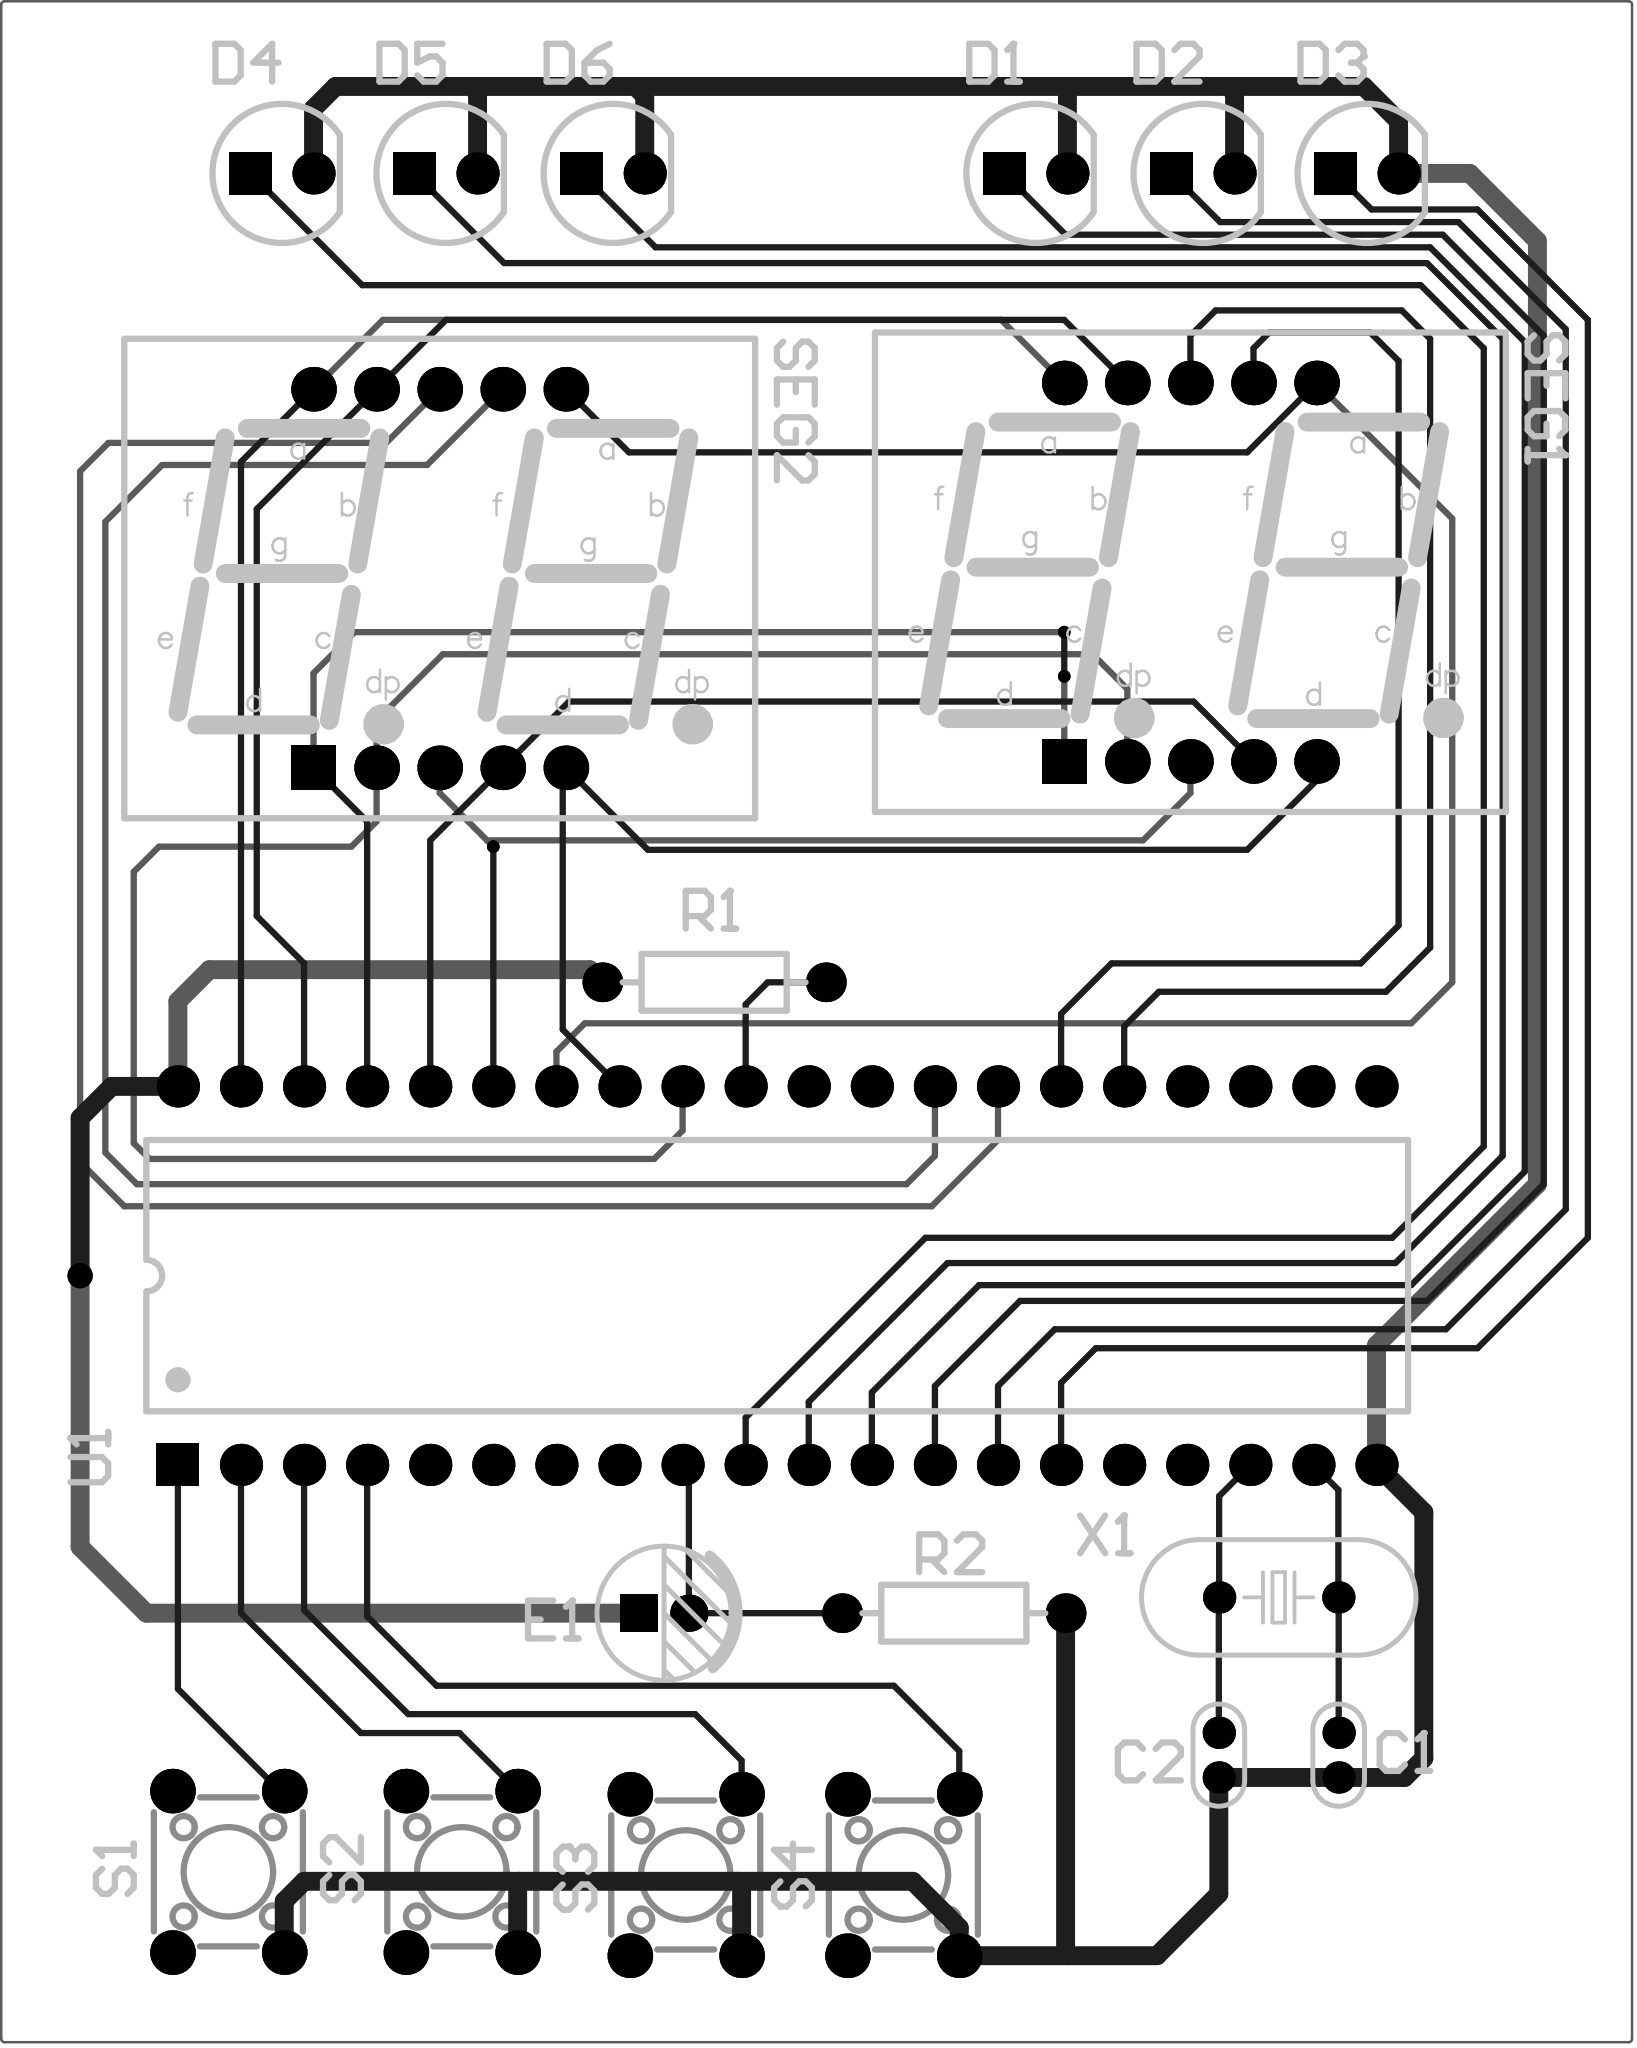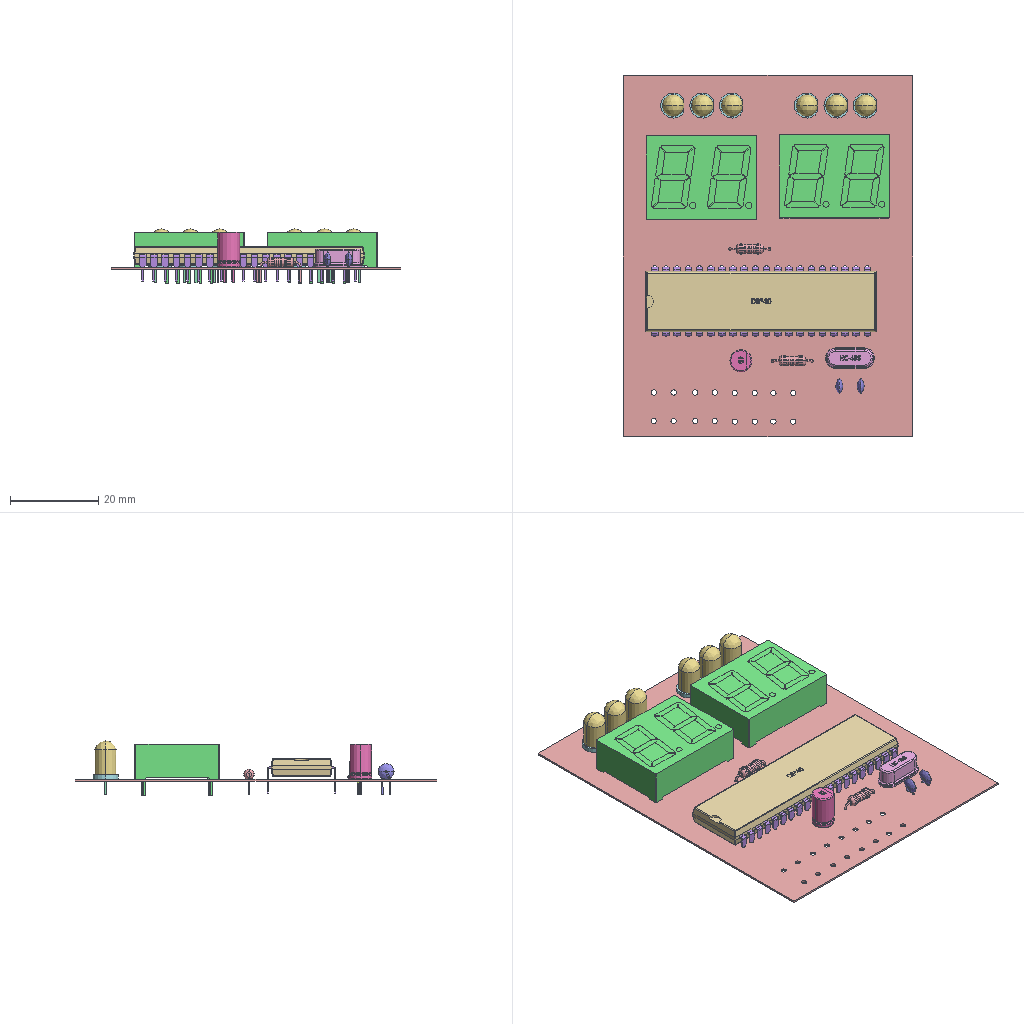Circuit board layout | Altium Designer | box 65.7 x 82.2 x 12.3 mm
Layer stack:
# Altium Designer layer stack of  (unit mm; dielectric type: 0 none, 1 core, 2 prepreg, 3 surface material)
index,name,kind,layer,copper_thickness_mm,dielectric_type,dielectric_thickness_mm,dielectric_material,dielectric_constant
0,Top Paste,other,,,,,,
1,Top Overlay,other,,,,,,
2,Top Solder,dielectric,,,3,0.0102,Solder Resist,3.5
3,Top Layer,copper,Top Layer,0.0356,,,,
4,Dielectric 1,dielectric,,,0,0.32,FR-4,4.8
5,Bottom Layer,copper,Bottom Layer,0.0356,,,,
6,Bottom Solder,dielectric,,,3,0.0102,Solder Resist,3.5
7,Bottom Overlay,other,,,,,,
8,Bottom Paste,other,,,,,,
# drill layer pairs: low layer,high layer
drill_pair,Top Layer,Bottom Layer
Part placement:
Designator,Comment,Layer,Footprint,Center-X(mm),Center-Y(mm),Rotation
X1,12MHz,TopLayer,OSC_HC-49S,103.505,45.212,360
U1,AT89C52,TopLayer,DIP40,83.312,58.166,90
SEG2,0.56IN-2-K,TopLayer,0.56IN-2P,69.723,86.233,360
SEG1,0.56IN-2-K,TopLayer,0.56IN-2P,99.949,86.487,360
S4,Plus,TopLayer,四脚轻触开关,88.392,34.036,270
S3,Minus,TopLayer,四脚轻触开关,79.629,34.036,270
S2,Set red,TopLayer,四脚轻触开关,70.612,34.163,270
S1,Set green,TopLayer,四脚轻触开关,61.214,34.163,270
R2,10K,TopLayer,RS_1/4W,90.424,44.577,180
R1,4.7K,TopLayer,RS_1/4W,80.772,69.977,360
E1,33PF,TopLayer,CS_2.0*5*8_-_C,78.756,44.577,180
D6,LED,TopLayer,LED_5MM-W,76.708,102.544,0
D5,LED,TopLayer,LED_5MM-W,69.977,102.544,0
D4,LED,TopLayer,LED_5MM-W,63.373,102.544,0
D3,LED,TopLayer,LED_5MM-W,107.061,102.544,0
D2,LED,TopLayer,LED_5MM-W,100.457,102.544,0
D1,LED,TopLayer,LED_5MM-W,93.726,102.544,0
C2,30PF,TopLayer,CC_1.8*3.6,101.092,38.862,90
C1,30PF,TopLayer,CC_1.8*3.6,105.918,38.862,90
Pad and via stacks:
# Altium Designer via and pad stacks of  (unit mm). Each distinct definition once, with the count of objects using it.
# via: kind,start_layer,end_layer,hole_mm,diameter_mm,mode(0 simple;1 top-mid-bottom;2 full stack),diameter_per_layer,count,example_net
# pad: kind,layer,hole_mm,hole_type(0 round;1 square;2 slot),plating,top_size,top_shape(1 round;2 rect;3 octagon;9 rounded rect),mid_size,bottom_size,mode,footprint,size_per_layer,count,example
pad,Multi-Layer,1.2,0,plated,1.8x1.8,1,1.8x1.8,1.8x1.8,0,\u00CB\u00C4\u00BD\u00C5\u00C7\u00E1\u00B4\u00A5\u00BF\u00AA\u00B9\u00D8,,16,S1.1
pad,Multi-Layer,0.8,0,plated,1.7x1.7,1,1.7x1.7,1.7x1.7,0,DIP40,,39,U1.21
pad,Multi-Layer,0.8,0,plated,1.7x1.7,2,1.7x1.7,1.7x1.7,0,DIP40,,1,U1.1
pad,Multi-Layer,0.6,0,plated,1.6x1.6,1,1.6x1.6,1.6x1.6,0,RS 1/4W,,4,R1.2
pad,Multi-Layer,0.5,0,plated,1.3x1.3,1,1.3x1.3,1.3x1.3,0,CC 1.8*3.6,,4,C1.2
pad,Multi-Layer,0.6,0,plated,1.3x1.3,1,1.3x1.3,1.3x1.3,0,OSC HC-49S,,2,X1.2
pad,Multi-Layer,0.8,0,plated,1.5x1.5,2,1.5x1.5,1.5x1.5,0,CS 2.0*5*8 - C,,1,E1.1
pad,Multi-Layer,0.8,0,plated,1.5x1.5,1,1.5x1.5,1.5x1.5,0,CS 2.0*5*8 - C,,1,E1.2
pad,Multi-Layer,0.9,0,plated,1.7x1.7,1,1.7x1.7,1.7x1.7,0,LED 5MM-W,,6,D3.2
pad,Multi-Layer,0.9,0,plated,1.7x1.7,2,1.7x1.7,1.7x1.7,0,LED 5MM-W,,6,D3.1
pad,Multi-Layer,0.9,0,plated,1.8x1.8,2,1.8x1.8,1.8x1.8,0,0.56IN-2P,,2,SEG1.1
pad,Multi-Layer,0.9,0,plated,1.8x1.8,1,1.8x1.8,1.8x1.8,0,0.56IN-2P,,18,SEG1.2
via,Top Layer,Bottom Layer,0.508,1.016,0,,1,+5V
via,Top Layer,Bottom Layer,0.254,0.508,0,,3,E
Design rules, without the lines most boards share:
# Altium Designer design rules of  (exported by Altium Designer, unit mm)
# columns: name | kind | enabled | priority | scope1 | scope2 | descriptor | typed fields (field=value)
SilkToSilkClearance | 55 | enabled | 1 | All | All | Silk to Silk (Clearance=0mil) (All),(All) |
SilkToSolderMaskClearance | 54 | enabled | 1 | IsPad | All | Silk To Solder Mask (Clearance=0mil) (IsPad),(All) |
MinimumSolderMaskSliver | 53 | enabled | 1 | All | All | Minimum Solder Mask Sliver (Gap=0mil) (All),(All) |
HoleToHoleClearance | 52 | enabled | 1 | All | All | Hole To Hole Clearance (Gap=10mil) (All),(All) | gap=0.254
DiffPairsRouting | 51 | enabled | 1 | All | All | Differential Pairs Uncoupled Length using the Gap Constraints (Min=10mil) (Max=10mil) (Prefered=10mil)  and Width Constraints (Min=15mil) (Max=15mil) (Prefered=15mil) (All) |
SolderMaskExpansion | 13 | enabled | 1 | All | All | Solder Mask Expansion (Expansion =4mil) (All) | expansion=0.1016
PasteMaskExpansion | 14 | enabled | 1 | All | All | Paste Mask Expansion (Expansion =0mil) (All) | expansion=0
RoutingVias | 11 | enabled | 1 | All | All | Routing Via (MinHoleWidth=28mil) (MaxHoleWidth=28mil) (PreferredHoleWidth=28mil) (MinWidth=50mil) (MaxWidth=50mil) (PreferedWidth=50mil) (All) | via_min_hole=0.7112 via_max_hole=0.7112 via_preferred_diameter=1.27 via_preferred_hole=0.7112
Width | 2 | enabled | 1 | All | All | Width Constraint (Min=10mil) (Max=30mil) (Preferred=10mil) (All) |
PolygonConnect | 20 | enabled | 1 | All | All | Polygon Connect Rule(Relief Connect )(Conductor Width=10mil) (Relief Angle=90 Angle) (Entries=4) (Air Gap Width=10mil) (All),(All) | connect_style(0=relief,1=direct,2=none)=0 relief_conductor_width=0.254 relief_entries=4
PlaneConnect | 6 | enabled | 1 | All | All | Power Plane Connect Rule(Relief Connect )(Expansion=20mil) (Conductor Width=10mil) (Air Gap=10mil) (Entries=4) (All) | relief_conductor_width=0.254 relief_entries=4 relief_expansion=0.508
Clearance | 0 | enabled | 1 | All | All | Clearance Constraint (Gap=10mil) (All),(All) | gap=0.254
Classes set for this board:
# Altium Designer classes of  (member kind: 0 net, 1 component, 2 from-to, 3 pad, 4 layer, 5 differential pair, 6 design channel, 7 polygon, 8 structure, 9 xSignal)
# columns: class name | member kind | superclass | members
Sheet1 | 1 | no | C1; C2; D1; D2; D3; D4; D5; D6; E1; R1; R2; S1; S2; S3; S4; SEG1; SEG2; U1; X1;